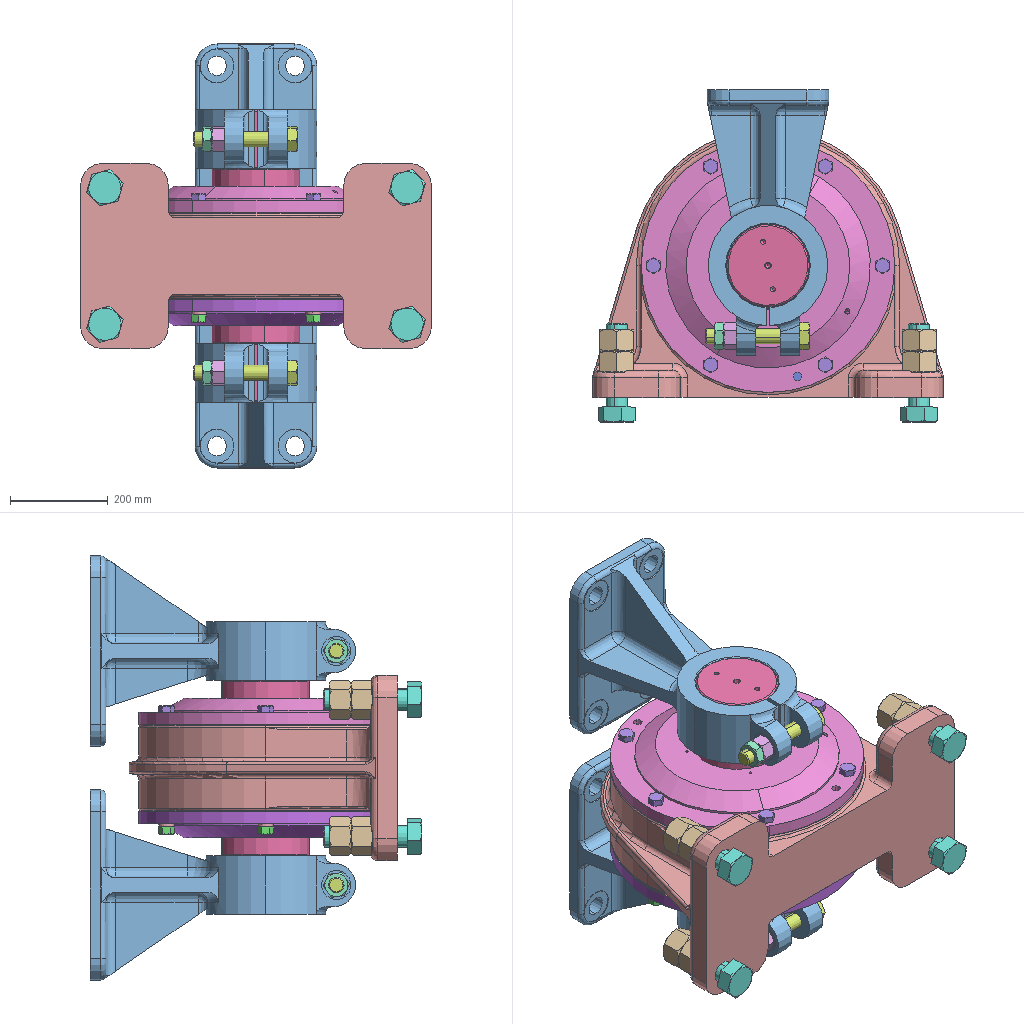Assembly | SolidWorks | 17 different items | 49 placed | box 720 x 680 x 870 mm
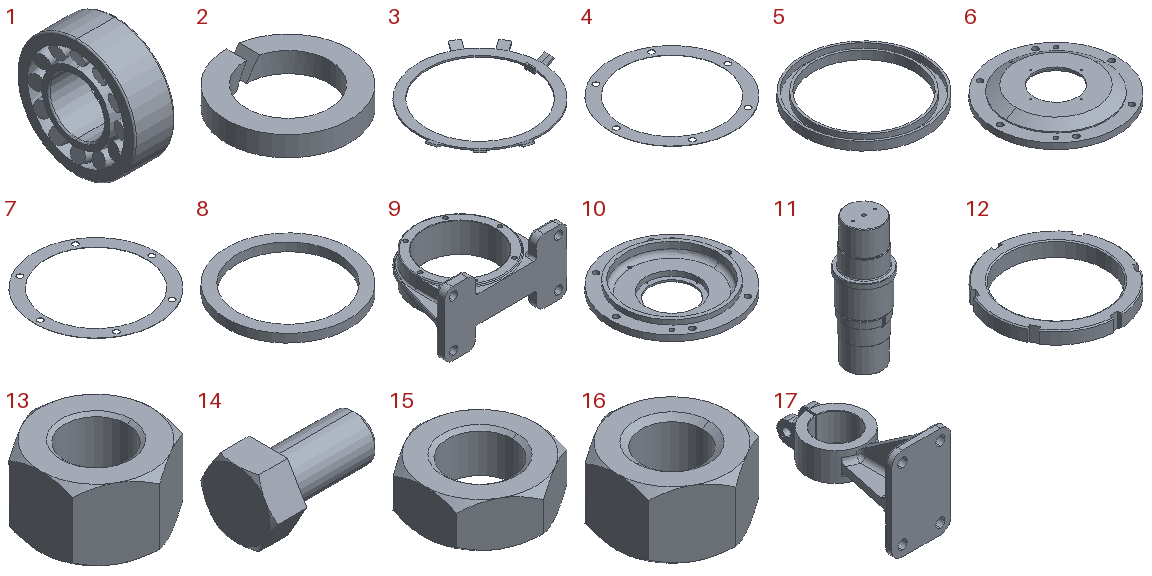Parts list (item | quantity | size | volume | features):
1 | x1 | 102 x 300 x 300 mm | 3829439 mm3 | features Revolution 4, Fillet 2, CirPattern 1, MirrorPattern 1, MirrorSolid 1
2 | x6 | 22.1 x 22.1 x 3.6 mm | 726.172 mm3 | features Cut 1, Extrusion 1
3 | x1 | 223.898 x 212.404 x 8.087 mm | 24578 mm3 | features Boss 1, Cut 1, Revolution 1
4 | x1 | 519 x 519 x 1 mm | 69858 mm3 | features CirPattern 1, Extrusion 1, ICE 1
5 | x1 | 220 x 220 x 15 mm | 105558 mm3 | features Extrusion 1, Shell 1
6 | x1 | 520 x 520 x 74 mm | 4938008 mm3 | features MirrorStock 1
7 | x1 | 519 x 519 x 1 mm | 69858 mm3 | features MirrorStock 1
8 | x1 | 220 x 220 x 15 mm | 105558 mm3 | features MirrorStock 1
9 | x1 | 720 x 550 x 380 mm | 24618968 mm3 | features Fillet 10, ICE 6, Chamfer 1, CirPattern 1, Extrusion 1, LPattern 1
10 | x1 | 520 x 520 x 74 mm | 4938016 mm3 | features CirPattern 3, HoleWzd 2, ICE 2, 3DProfileFeature 1, Fillet 1, Revolution 1
11 | x1 | 220 x 220 x 600 mm | 15781645 mm3 | features ICE 9, Chamfer 4, HoleWzd 3, Fillet 2, Extrusion 1, MirrorPattern 1
12 | x1 | 240 x 239.437 x 30 mm | 460595 mm3 | features Chamfer 3, CirPattern 1, Cut 1, Extrusion 1
13 | x8 | 69.85 x 80.656 x 44.679 mm | 131935 mm3 | features RevCut 4, Extrusion 1, LPattern 1
14 | x12 | 25.857 x 16.483 x 14.275 mm | 2543 mm3 | features RevCut 2, Extrusion 1, Fillet 1, LPattern 1, Revolution 1
15 | x2 | 47.625 x 54.993 x 19.075 mm | 25013 mm3 | features RevCut 4, Extrusion 1, LPattern 1
16 | x8 | 14.275 x 16.483 x 8.56 mm | 1065 mm3 | features RevCut 4, Extrusion 1, LPattern 1
17 | x2 | 250 x 545 x 390 mm | 8795912 mm3 | features ICE 9, Fillet 7, Chamfer 1, Extrusion 1, LPattern 1
Mates (type | each side: item.copy, entity, surface, feature):
Coincident | 9.1 plane | assembly plane | 3 times
Coincident | 1.1 plane | assembly plane
Concentric | 9.1 face cylinder Boss-Extrude1 | 1.1 face cylinder Revolve3
Coincident | 1.1 face plane Revolve1 | 11.1 face plane Boss-Extrude2
Concentric | 1.1 face cylinder Revolve1 | 11.1 face cylinder Boss-Extrude1
Coincident | 1.1 face plane Revolve1 | 3.1 face plane Base-Extrude
Concentric | 3.1 face cylinder Cut-Extrude | 11.1 face cylinder Boss-Extrude5
Coincident | 3.1 face plane Base-Extrude | 12.1 face plane Base-Extrude
Concentric | 11.1 face cylinder Boss-Extrude5 | 12.1 face cylinder Base-Extrude
Coincident | 10.1 face plane Revolve1 | 5.1 face plane Boss-Extrude1
Concentric | 10.1 face cylinder Revolve1 | 5.1 face cylinder Boss-Extrude1
Coincident | 10.1 face plane Revolve1 | 4.1 face plane Boss-Extrude1
Concentric | 10.1 face cylinder Revolve1 | 4.1 face cylinder Boss-Extrude1
Concentric | 10.1 face cylinder CirPattern2 | 4.1 face cylinder CirPattern1
Coincident | 1.1 face plane Revolve3 | 10.1 face plane Revolve1
Concentric | 11.1 face cylinder Boss-Extrude6 | 10.1 face cylinder Revolve1
Concentric | 9.1 face cylinder CirPattern1 | 10.1 face cylinder CirPattern2
Concentric | 9.1 face cylinder LPattern1 | 14.1 face cylinder BaseBody
DistanceDim | 14.1 face plane BaseHead | 9.1 face plane Boss-Extrude2
Coincident | 9.1 face plane LPattern1 | 13.1 face plane BaseNut
Concentric | 14.1 face cylinder BaseBody | 13.1 face cylinder BaseNut
Coincident | 13.1 face plane BaseNut | 13.2 face plane BaseNut
Concentric | 14.1 face cylinder BaseBody | 13.2 face cylinder BaseNut
Coincident | 6.1 face plane 640.01.51.03A Bearing coverMirror | 14.2 face plane BaseHead
Concentric | 6.1 face cylinder 640.01.51.03A Bearing coverMirror | 14.2 face cylinder BaseBody
Coincident | 10.1 face plane Revolve1 | 2.1 face plane Base-Extrude
Concentric | 14.2 face cylinder BaseBody | 2.1 face cylinder Base-Extrude
Coincident | 16.1 face plane BaseNut | 2.1 face plane Base-Extrude
Concentric | 14.2 face cylinder BaseBody | 16.1 face cylinder BaseNut
Coincident | 11.1 face plane Boss-Extrude3 | 17.1 face plane Boss-Extrude1
Concentric | 11.1 face cylinder Boss-Extrude8 | 17.1 face cylinder Boss-Extrude1
Coincident | 17.1 face plane Cut-Extrude2 | 14.3 face plane BaseHead
Concentric | 17.1 face cylinder Boss-Extrude5 | 14.3 face cylinder BaseBody
Coincident | 17.1 face plane Cut-Extrude1 | 16.2 face plane BaseNut
Concentric | 14.3 face cylinder BaseBody | 16.2 face cylinder BaseNut
Coincident | 16.2 face plane BaseNut | 15.1 face plane BaseNut
Concentric | 14.3 face cylinder BaseBody | 15.1 face cylinder BaseNut
Coincident | assembly plane | 17.1 plane